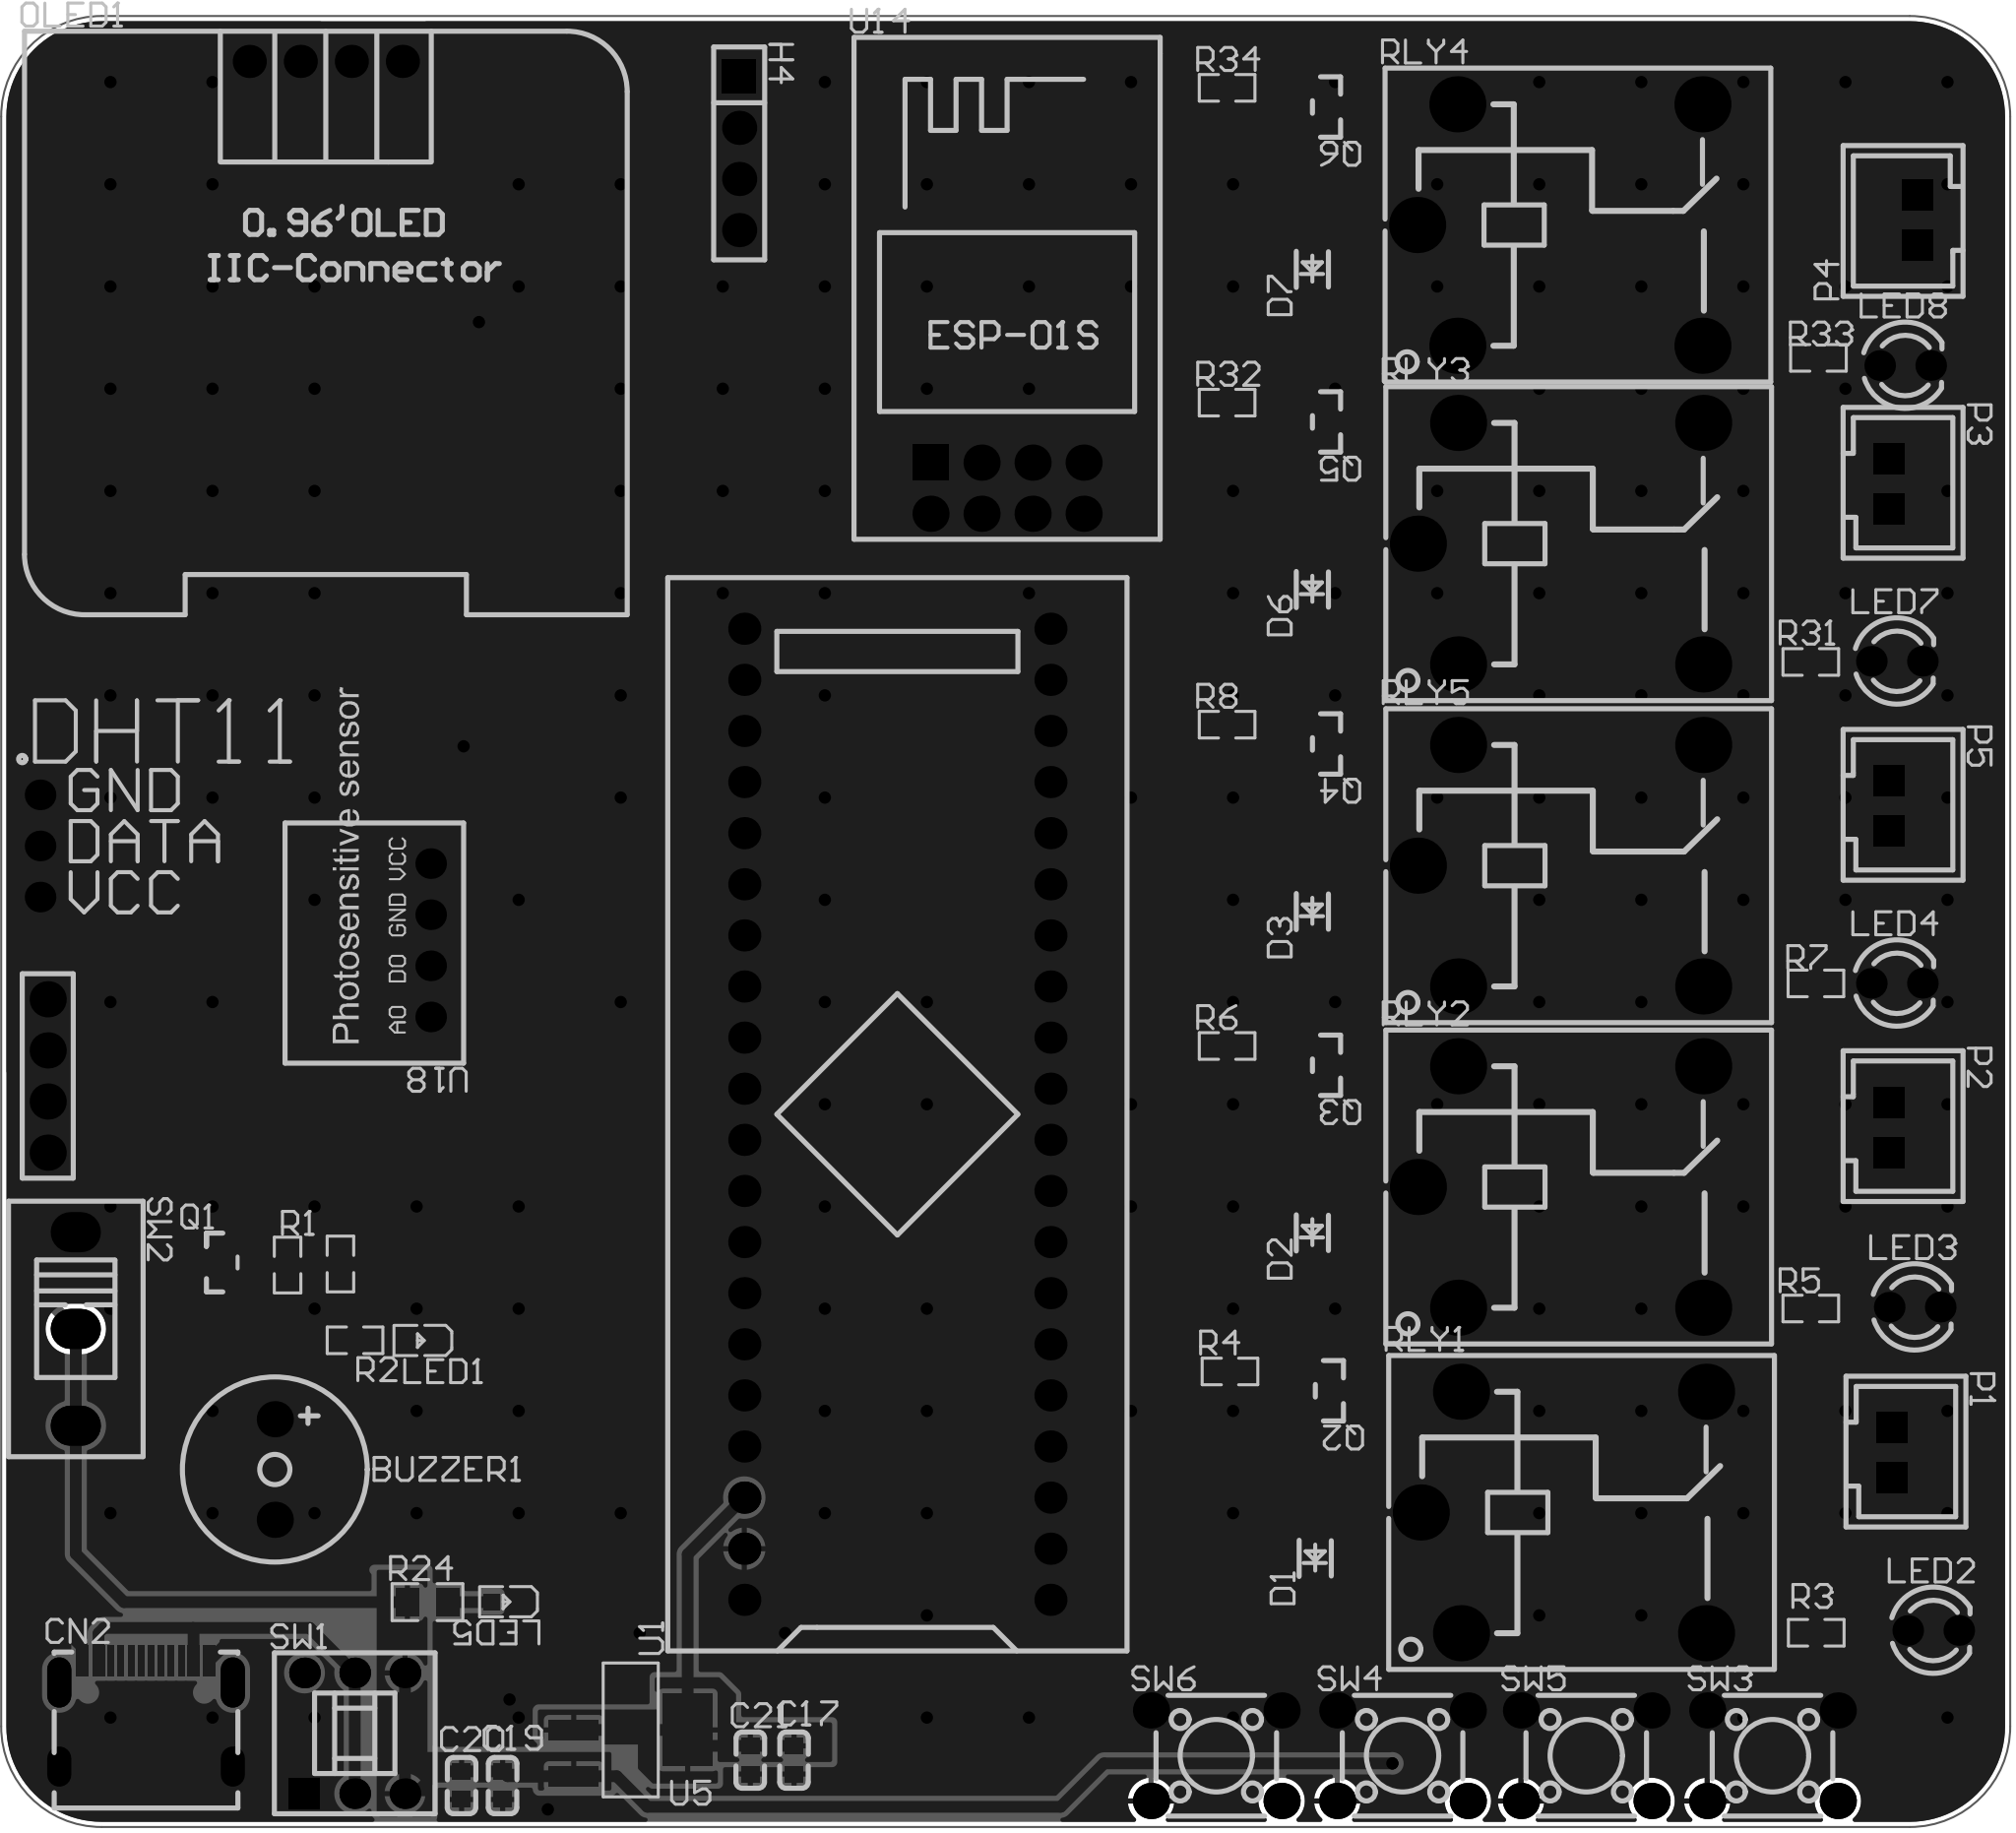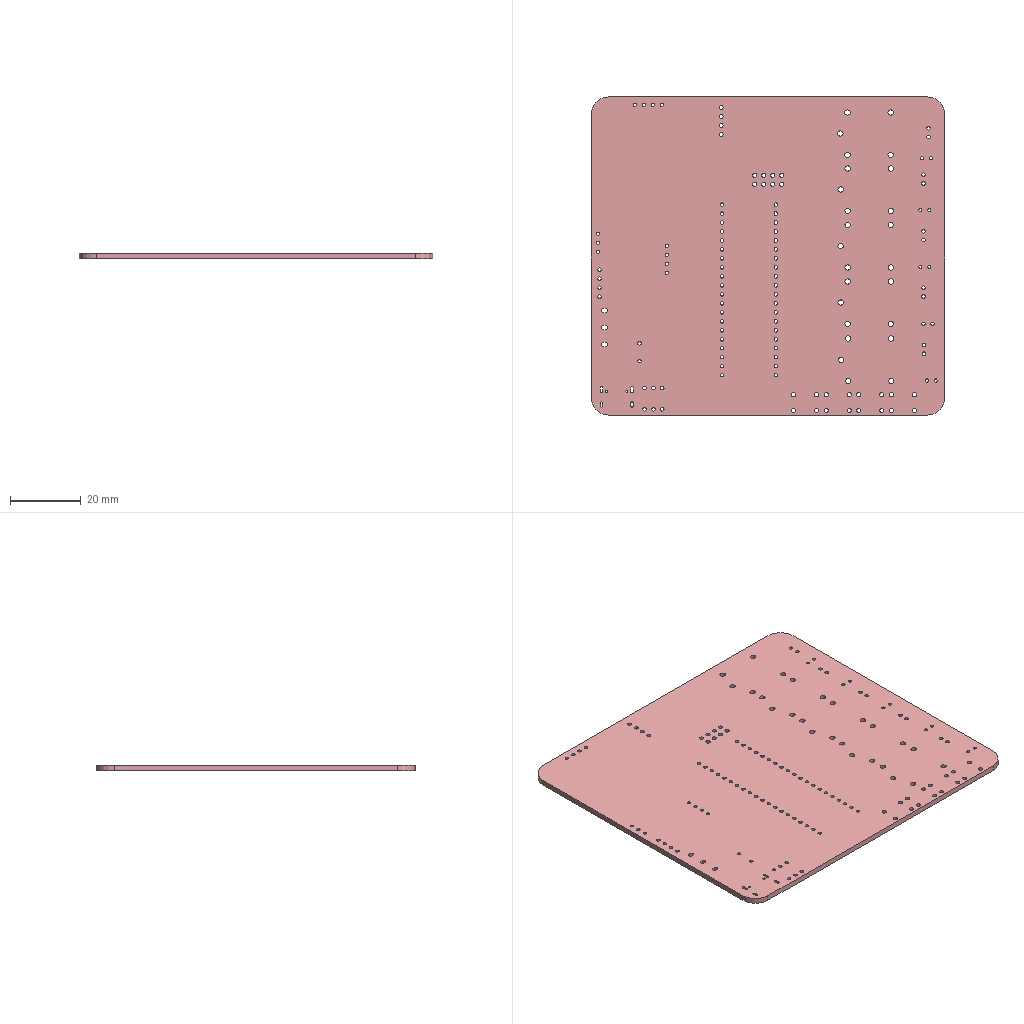Circuit board layout | Altium Designer | box 100 x 90 x 1.6 mm
Layer stack:
# Altium Designer layer stack of  (unit mm; dielectric type: 0 none, 1 core, 2 prepreg, 3 surface material)
index,name,kind,layer,copper_thickness_mm,dielectric_type,dielectric_thickness_mm,dielectric_material,dielectric_constant
0,Top Paste Mask Layer,other,,,,,,
1,Top Silkscreen Layer,other,,,,,,
2,Top Solder Mask Layer,dielectric,,,3,0.01,,3.3
3,Top Layer,copper,Top Layer,0.035,,,,
4,Dielectric1,dielectric,,,3,1.51,FR4,4.5
5,Bottom Layer,copper,Bottom Layer,0.035,,,,
6,Bottom Solder Mask Layer,dielectric,,,3,0.01,,3.3
7,Bottom Silkscreen Layer,other,,,,,,
8,Bottom Paste Mask Layer,other,,,,,,
# drill layer pairs: low layer,high layer
drill_pair,Top Layer,Bottom Layer
Part placement:
Designator,Comment,Layer,Footprint,Center-X(mm),Center-Y(mm),Rotation
CN2,USB-TYPEC,TopLayer,USB-C-SMD_MC-307,100.742,85.688,0
R28,1k,TopLayer,R0603,110.417,108.025,270
R24,4.7k,TopLayer,R0805,114.75,91.221,0
C20,10u,TopLayer,C0603,116.45,82.112,90
LED5,,TopLayer,LED_0603,118.734,91.246,180
C19,100n,TopLayer,C0603,118.492,82.112,90
U5,TLV1117LV33DCYT,TopLayer,SOT-223-4_L6.5-W3.5-P2.30-LS7.0-BR,124.866,84.87,180
C21,22u,TopLayer,C0603,130.821,83.379,90
C17,100n,TopLayer,C0603,132.998,83.379,90
R34,1k,TopLayer,R0603,154.552,166.475,0
R32,1k,TopLayer,R0603,154.552,150.832,0
Q6,,TopLayer,S8050_SOT-23,159.5,165.524,180
Q5,,TopLayer,S8050_SOT-23,159.5,149.874,180
D7,LL4148,TopLayer,LL-34_L3.5-W1.5-RD,158.795,157.454,90
D6,LL4148,TopLayer,LL-34_L3.5-W1.5-RD,158.795,141.543,90
R33,3.3k,TopLayer,R0603,183.986,153.057,0
R31,3.3k,TopLayer,R0603,183.605,137.944,0
U20,,TopLayer,dht11温湿度传感器,95.467,128.8,0
U18,Light intensity module,TopLayer,光敏传感器,114.91,124.113,180
U14,ESP-01S,TopLayer,WIFIM-TH_ESP-01S,143.6,146.58,0
BUZZER1,HNB09A03,TopLayer,BUZ-TH_BD9.0-P5.00-D0.6-FD,107.152,97.812,270
U19,,TopLayer,4P排母,95.848,117.37,270
SW1,K8-8081D-NNW,TopLayer,SW-TH_6P-L8.0-W8.0-P2.50,111.13,84.703,0
U1,LCKFB-DKX-STM32F103C8T6,TopLayer,CONN-TH_L53.3-W22.9_STM32F103C8T6-CARD,138.139,115.465,90
RLY4,SRD-05VDC-SL-C,TopLayer,RELAY-TH_SRD-XXVDC-XL-C,171.113,159.658,0
RLY3,SRD-05VDC-SL-C,TopLayer,RELAY-TH_SRD-XXVDC-XL-C,171.151,143.824,0
LED8,,TopLayer,LED_TH-3mm,188.304,152.676,0
LED7,,TopLayer,LED_TH-3mm,187.89,137.979,0
P3,XH2.54 straight socket 2P,TopLayer,CONN-TH_XH2.54-2P,187.5,146.786,270
P4,XH2.54 straight socket 2P,TopLayer,CONN-TH_XH2.54-2P,188.897,159.924,90
LED1,,TopLayer,LED_0603,114.471,104.231,180
Q1,,TopLayer,S8550P_SOT,104.399,108.099,0
R1,10k,TopLayer,R0603,107.786,107.972,270
R2,1k,TopLayer,R0603,111.144,104.233,180
SW3,,TopLayer,SW-TH_4P-L6.0-W6.0-P4.50-LS6.5,181.7,83.588,0
SW4,,TopLayer,SW-TH_4P-L6.0-W6.0-P4.50-LS6.5,163.285,83.588,0
SW5,,TopLayer,SW-TH_4P-L6.0-W6.0-P4.50-LS6.5,172.429,83.588,0
SW6,,TopLayer,SW-TH_4P-L6.0-W6.0-P4.50-LS6.5,154.014,83.588,0
SW2,XY-SS12D10L3,TopLayer,SW-TH_3P-L12.7-W6.7_XY-SS12D10LXX,97.245,104.797,270
D1,LL4148,TopLayer,LL-34_L3.5-W1.5-RD,158.938,93.396,90
D2,LL4148,TopLayer,LL-34_L3.5-W1.5-RD,158.795,109.57,90
D3,LL4148,TopLayer,LL-34_L3.5-W1.5-RD,158.795,125.538,90
LED2,,TopLayer,LED_TH-3mm,189.701,89.811,0
LED3,,TopLayer,LED_TH-3mm,188.779,105.879,0
LED4,,TopLayer,LED_TH-3mm,187.89,121.974,0
P1,XH2.54 straight socket 2P,TopLayer,CONN-TH_XH2.54-2P,187.643,98.638,270
P2,XH2.54 straight socket 2P,TopLayer,CONN-TH_XH2.54-2P,187.5,114.813,270
P5,XH2.54 straight socket 2P,TopLayer,CONN-TH_XH2.54-2P,187.5,130.781,270
Q2,,TopLayer,S8050_SOT-23,159.643,101.727,180
Q3,,TopLayer,S8050_SOT-23,159.5,117.901,180
Q4,,TopLayer,S8050_SOT-23,159.5,133.869,180
R3,3.3k,TopLayer,R0603,183.877,89.7,0
R4,1k,TopLayer,R0603,154.696,102.685,0
R5,3.3k,TopLayer,R0603,183.605,105.813,0
R6,1k,TopLayer,R0603,154.552,118.859,0
R7,3.3k,TopLayer,R0603,183.86,121.969,0
R8,1k,TopLayer,R0603,154.552,134.827,0
RLY1,SRD-05VDC-SL-C,TopLayer,RELAY-TH_SRD-XXVDC-XL-C,171.294,95.677,0
RLY2,SRD-05VDC-SL-C,TopLayer,RELAY-TH_SRD-XXVDC-XL-C,171.151,111.852,0
RLY5,SRD-05VDC-SL-C,TopLayer,RELAY-TH_SRD-XXVDC-XL-C,171.151,127.82,0
OLED1,,TopLayer,0.96OLED_4P,109.691,167.79,0
H4,,TopLayer,HDR-TH_4P-P2.54-V-F,130.265,163.217,270
Pad and via stacks:
# Altium Designer via and pad stacks of  (unit mm). Each distinct definition once, with the count of objects using it.
# via: kind,start_layer,end_layer,hole_mm,diameter_mm,mode(0 simple;1 top-mid-bottom;2 full stack),diameter_per_layer,count,example_net
# pad: kind,layer,hole_mm,hole_type(0 round;1 square;2 slot),plating,top_size,top_shape(1 round;2 rect;3 octagon;9 rounded rect),mid_size,bottom_size,mode,footprint,size_per_layer,count,example
pad,Top Layer,0,0,plated,0.6x1.524,2,0.6x1.524,0.6x1.524,0,USB-C-SMD_MC-307,,4,CN2.A1B12
pad,Top Layer,0,0,plated,0.3x1.524,2,0.3x1.524,0.3x1.524,0,USB-C-SMD_MC-307,,8,CN2.B5
pad,Top Layer,0,0,plated,0.8065x0.864,2,0.8065x0.864,0.8065x0.864,0,R0603,,26,R28.2
pad,Top Layer,0,0,plated,1.133x1.377,2,1.133x1.377,1.133x1.377,0,R0805,,2,R24.2
pad,Top Layer,0,0,plated,0.8x0.9,2,0.8x0.9,0.8x0.9,0,C0603,,8,C20.2
pad,Top Layer,0,0,plated,0.8001x0.8001,2,0.8001x0.8001,0.8001x0.8001,0,LED_0603,,4,LED5.1
pad,Top Layer,0,0,plated,2.47x0.98,2,2.47x0.98,2.47x0.98,0,SOT-223-4_L6.5-W3.5-P2.30-LS7.0-BR,,3,U5.1
pad,Top Layer,0,0,plated,2.47x3.6,2,2.47x3.6,2.47x3.6,0,SOT-223-4_L6.5-W3.5-P2.30-LS7.0-BR,,1,U5.4
pad,Top Layer,0,0,plated,1x0.8,2,1x0.8,1x0.8,0,S8050_SOT-23,,15,Q6.2
pad,Top Layer,0,0,plated,1.1x1.7,2,1.1x1.7,1.1x1.7,0,LL-34_L3.5-W1.5-RD,,10,D7.2
pad,Top Layer,0,0,plated,0.701x1.25,2,0.701x1.25,0.701x1.25,0,S8550P_SOT,,3,Q1.3
pad,Multi-Layer,0.7,2,plated,1.2x2,1,1.2x2,1.2x2,0,USB-C-SMD_MC-307,,2,CN2.0
pad,Multi-Layer,0.7,2,plated,1.2x2.5,1,1.2x2.5,1.2x2.5,0,USB-C-SMD_MC-307,,2,CN2.2
pad,Multi-Layer,0.9144,0,plated,1.524x1.524,1,1.524x1.524,1.524x1.524,0,dht11\u00CE\u00C2\u00CA\u00AA\u00B6\u00C8\u00B4\u00AB\u00B8\u00D0\u00C6\u00F7,,3,U20.1
pad,Multi-Layer,0.9144,2,plated,1.524x1.524,1,1.524x1.524,1.524x1.524,0,\u00B9\u00E2\u00C3\u00F4\u00B4\u00AB\u00B8\u00D0\u00C6\u00F7,,4,U18.1
pad,Multi-Layer,1.2,0,plated,1.8x1.8,2,1.8x1.8,1.8x1.8,0,WIFIM-TH_ESP-01S,,1,U14.1
pad,Multi-Layer,1.2,0,plated,1.8x1.8,1,1.8x1.8,1.8x1.8,0,WIFIM-TH_ESP-01S,,7,U14.2
pad,Multi-Layer,1,0,plated,1.8x1.8,1,1.8x1.8,1.8x1.8,0,BUZ-TH_BD9.0-P5.00-D0.6-FD,,2,BUZZER1.1
pad,Multi-Layer,1,0,plated,1.8x1.8,1,1.8x1.8,1.8x1.8,0,4P\u00C5\u00C5\u00C4\u00B8,,4,U19.1
pad,Multi-Layer,1,0,plated,1.524x1.524,1,1.524x1.524,1.524x1.524,0,SW-TH_6P-L8.0-W8.0-P2.50,,5,SW1.3
pad,Multi-Layer,1,0,plated,1.524x1.524,2,1.524x1.524,1.524x1.524,0,SW-TH_6P-L8.0-W8.0-P2.50,,1,SW1.1
pad,Multi-Layer,1,0,plated,1.6x1.6,1,1.6x1.6,1.6x1.6,0,CONN-TH_L53.3-W22.9_STM32F103C8T6-CARD,,40,U1.1
pad,Multi-Layer,1.524,0,plated,2.794x2.794,1,2.794x2.794,2.794x2.794,0,RELAY-TH_SRD-XXVDC-XL-C,,25,RLY4.2
pad,Multi-Layer,0.9144,0,plated,1.524x1.524,1,1.524x1.524,1.524x1.524,0,LED_TH-3mm,,10,LED8.1
pad,Multi-Layer,1,2,plated,1.524x1.524,2,1.524x1.524,1.524x1.524,0,CONN-TH_XH2.54-2P,,10,P3.1
pad,Multi-Layer,1.2,0,plated,1.8x1.8,1,1.8x1.8,1.8x1.8,0,SW-TH_4P-L6.0-W6.0-P4.50-LS6.5,,16,SW3.1
pad,Multi-Layer,1.2,2,plated,2x2.5,1,2x2.5,2x2.5,0,SW-TH_3P-L12.7-W6.7_XY-SS12D10LXX,,3,SW2.1
pad,Multi-Layer,1,0,plated,1.65x1.65,1,1.65x1.65,1.65x1.65,0,0.96OLED_4P,,4,OLED1.4
pad,Multi-Layer,1.1,0,plated,1.7x1.7,2,1.7x1.7,1.7x1.7,0,HDR-TH_4P-P2.54-V-F,,1,H4.1
pad,Multi-Layer,1.1,0,plated,1.7x1.7,1,1.7x1.7,1.7x1.7,0,HDR-TH_4P-P2.54-V-F,,3,H4.2
via,Top Layer,Bottom Layer,0.3048,0.61,0,,205,SDA
Copper pours:
name,layer,net,type(0 solid;1 hatched;2 none)
Bottom Layer-GND,Bottom Layer,GND,0
Top Layer-+5V,Top Layer,+5V,0
Top Layer-VCC,Top Layer,VCC,0
Top Layer-GND,Top Layer,GND,0